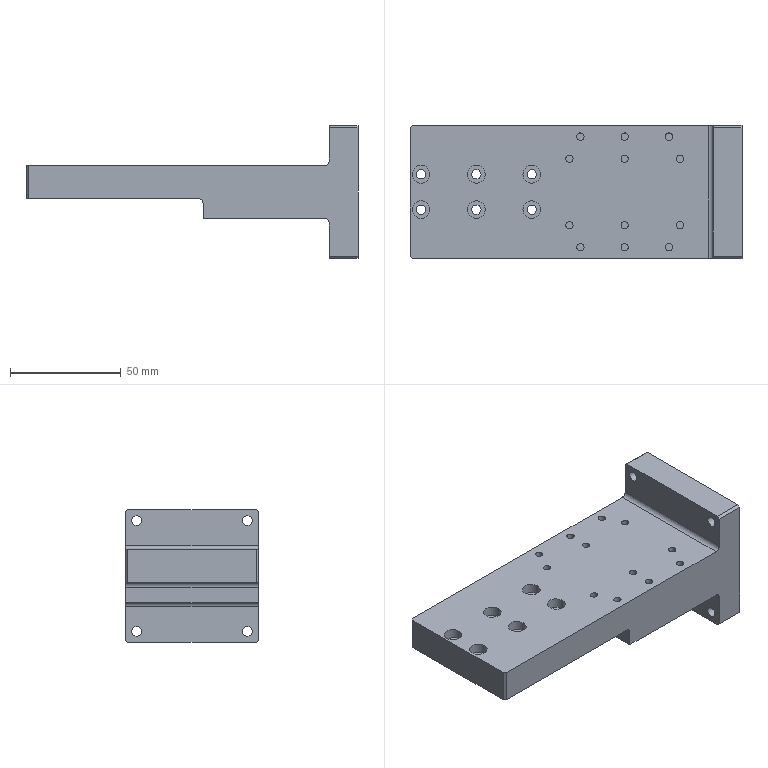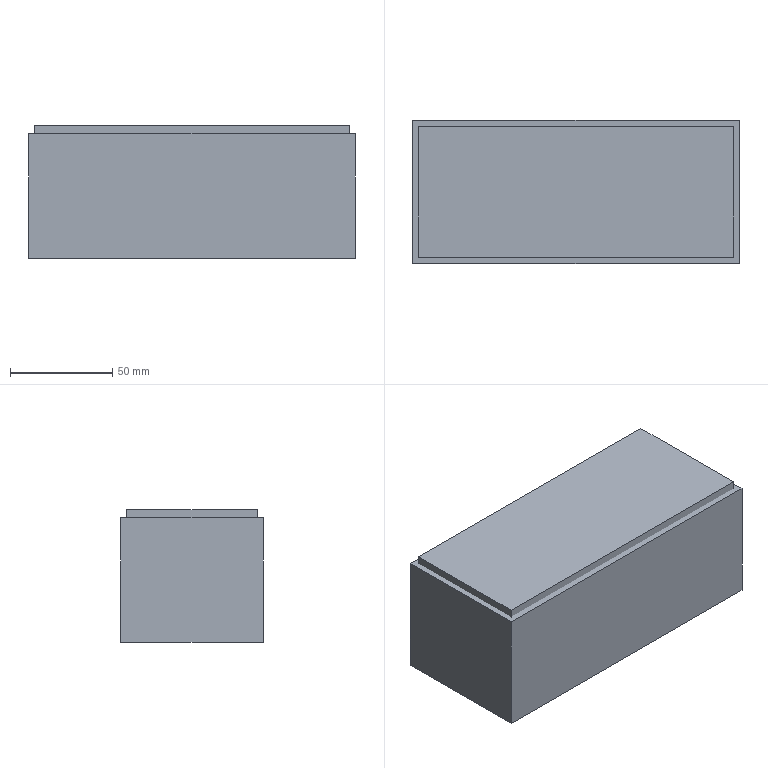CAM job | NX | 3+2 milling, drilling | part box 150 x 60 x 60 mm | stock box 160 x 70 x 65 mm
Tools:
number,name,description,diameter,corner_radius,flute_length,length,flutes
19,D80,Milling Tool-5 Parameters,80.0,0.0,50.0,75.0,2
15,D10,Milling Tool-5 Parameters,10.0,0.0,50.0,75.0,2
14,D10JING,Milling Tool-5 Parameters,10.0,0.0,50.0,75.0,2
5,D4R0.5,Milling Tool-5 Parameters,4.0,0.5,50.0,75.0,2
1,D6A45,Milling Tool-5 Parameters,6.0,0.0,50.0,75.0,2
3,3.3ZT,Drilling Tool,3.3,0.0,35.0,50.0,2
4,4.2ZT,Drilling Tool,4.2,0.0,35.0,50.0,2
12,D6,Milling Tool-5 Parameters,6.0,0.0,50.0,75.0,2
8,4.5ZT,Drilling Tool,4.5,0.0,35.0,50.0,2
Operations:
program,operation,operation_type,tool,method,geometry_group,spindle_rpm,surface_speed,feed_per_tooth,feed_cut,feed_plunge,cut_length_mm,path_length_mm,cut_time_min,machine_time_min
1,FLOOR_WALL,VolumeBased25DMillingOperation,D80,METHOD,A,6500.0,1633.0,0.1154,1500.0,100.0,252.0,306.0,0.168,0.1734
1,ADAPTIVE_MILLING,CavityMilling,D10,METHOD,A,9500.0,298.0,0.1579,3000.0,1000.0,9352.535,11581.463,3.135,3.358
1,FLOOR_WALL_1,VolumeBased25DMillingOperation,D10,METHOD,A,9500.0,298.0,0.1579,3000.0,1000.0,14688.71,14778.51,4.901,4.91
1,PLANAR_MILL,PlanarMilling,D10,METHOD,A,9500.0,298.0,0.1316,2500.0,1000.0,277.162,828.553,0.122,0.1772
1,ZLEVEL_PROFILE_COPY_1_COPY,ZLevelMilling,D10JING,METHOD,A,9500.0,298.0,0.0632,1200.0,1000.0,1374.708,1789.636,1.148,1.19
1,FLOOR_WALL_1_COPY,VolumeBased25DMillingOperation,D10JING,METHOD,A,9500.0,298.0,0.0789,1500.0,1000.0,2113.499,2369.501,1.413,1.439
1,ZLEVEL_PROFILE_COPY_1_COPY_COPY,ZLevelMilling,D10JING,METHOD,A,9500.0,298.0,0.0632,1200.0,1000.0,78.46,166.26,0.0663,0.0751
1,FIXED_CONTOUR,SurfaceContour,D4R0.5,METHOD,A,9500.0,119.0,0.1579,3000.0,100.0,1423.975,1479.175,0.4747,0.4802
1,DRILLING,Operation,D6A45,METHOD,A,5000.0,94.0,0.035,350.0,0.0,72.0,591.726,0.2057,0.2577
1,DRILLING_COPY_1,Operation,3.3ZT,METHOD,A,2000.0,20.0,0.05,200.0,0.0,167.897,647.697,0.8395,0.8875
1,DRILLING_COPY_1_COPY,Operation,4.2ZT,METHOD,A,2000.0,20.0,0.05,200.0,0.0,121.571,453.337,0.6079,0.641
1,HOLE_MILLING,CylinderMilling,D6,METHOD,A,9500.0,179.0,0.0868,1650.0,100.0,372.137,1079.5,0.2255,0.2963
1,PLANAR_MILL_COPY_COPY_COPY,PlanarMilling,D6A45,METHOD,A,9500.0,179.0,0.0658,1250.0,100.0,156.749,215.749,0.1254,0.1313
1,PLANAR_MILL_COPY_COPY_COPY_COPY,PlanarMilling,D6A45,METHOD,A,9500.0,179.0,0.0658,1250.0,100.0,639.133,2832.511,0.5113,0.7306
2,FLOOR_WALL_COPY,VolumeBased25DMillingOperation,D80,METHOD,B,6500.0,1633.0,0.1154,1500.0,100.0,1230.0,2440.001,0.82,0.941
2,FLOOR_WALL_1_COPY_1,VolumeBased25DMillingOperation,D10,METHOD,B,9500.0,298.0,0.1579,3000.0,1000.0,8542.684,8650.484,2.852,2.863
2,PLANAR_MILL_COPY,PlanarMilling,D10,METHOD,B,9500.0,298.0,0.1316,2500.0,1000.0,277.162,900.553,0.122,0.1844
2,FLOOR_WALL_1_COPY_1_COPY,VolumeBased25DMillingOperation,D10,METHOD,B,9500.0,298.0,0.1579,3000.0,1000.0,6086.975,6176.775,2.033,2.042
2,PLANAR_MILL_COPY_COPY,PlanarMilling,D10,METHOD,B,9500.0,298.0,0.1316,2500.0,1000.0,269.162,814.553,0.1188,0.1734
2,FLOOR_WALL_1_COPY_COPY,VolumeBased25DMillingOperation,D10JING,METHOD,B,9500.0,298.0,0.0789,1500.0,1000.0,2199.998,2823.084,1.475,1.537
2,ZLEVEL_PROFILE_COPY_1_COPY_COPY_COPY,ZLevelMilling,D10JING,METHOD,B,9500.0,298.0,0.0632,1200.0,1000.0,78.457,184.257,0.0663,0.0769
2,ZLEVEL_PROFILE_COPY_1_COPY_COPY_COPY_COPY,ZLevelMilling,D10JING,METHOD,B,9500.0,298.0,0.0632,1200.0,1000.0,78.459,166.259,0.0663,0.0751
2,FIXED_CONTOUR_COPY,SurfaceContour,D4R0.5,METHOD,B,9500.0,119.0,0.1579,3000.0,100.0,2890.142,3123.251,0.9634,0.9867
2,DRILLING_COPY,Operation,D6A45,METHOD,B,5000.0,94.0,0.035,350.0,0.0,16.0,305.27,0.0457,0.0746
2,DRILLING_COPY_1_COPY_1,Operation,3.3ZT,METHOD,B,2000.0,20.0,0.05,200.0,0.0,51.966,377.201,0.2598,0.2924
2,PLANAR_MILL_COPY_COPY_COPY_COPY_1,PlanarMilling,D6A45,METHOD,B,9500.0,179.0,0.0658,1250.0,100.0,152.749,211.749,0.1222,0.1281
2,PLANAR_MILL_COPY_COPY_COPY_COPY_COPY,PlanarMilling,D6A45,METHOD,B,9500.0,179.0,0.0658,1250.0,100.0,172.339,267.339,0.1379,0.1474
2,PLANAR_MILL_COPY_COPY_COPY_COPY_COPY_COPY,PlanarMilling,D6A45,METHOD,B,9500.0,179.0,0.0658,1250.0,100.0,362.652,1843.206,0.2901,0.4382
3,DRILLING_COPY_COPY,Operation,D6A45,METHOD,C,5000.0,94.0,0.035,350.0,0.0,21.4,262.07,0.0611,0.0852
3,DRILLING_COPY_1_COPY_1_COPY,Operation,4.5ZT,METHOD,C,2000.0,20.0,0.05,200.0,0.0,75.408,370.085,0.377,0.4065